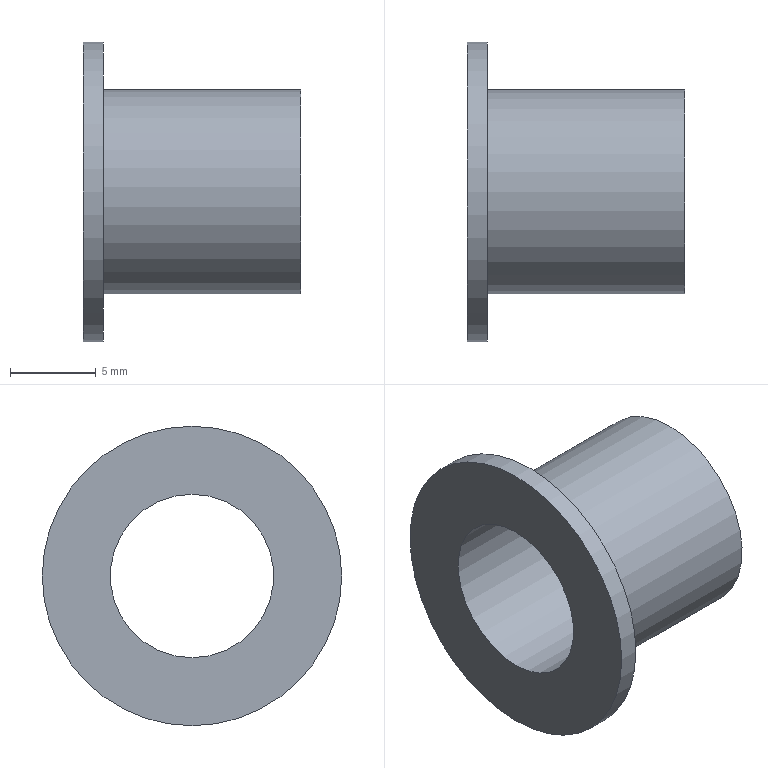Part | NX | features Igus GFI bushings(0.375 x 0.500) 2 | 1 solid | 6 faces | box 12.7 x 17.45 x 17.45 mm | volume 658.37 mm3 | plane 3 | cylinder 3 | commonest cylinder face diameters 9.525 x1 11.906 x1 17.45 x1
STEP:
#1=CARTESIAN_POINT('',(0.,0.,4.763));
#2=VERTEX_POINT('',#1);
#3=CARTESIAN_POINT('',(0.,0.,0.));
#4=DIRECTION('',(-1.,0.,0.));
#5=DIRECTION('',(0.,0.,1.));
#6=AXIS2_PLACEMENT_3D('',#3,#4,#5);
#7=CIRCLE('',#6,4.763);
#8=EDGE_CURVE('',#2,#2,#7,.T.);
#9=ORIENTED_EDGE('',*,*,#8,.F.);
#10=EDGE_LOOP('',(#9));
#11=FACE_BOUND('',#10,.T.);
#12=CARTESIAN_POINT('',(0.,0.,8.725));
#13=VERTEX_POINT('',#12);
#14=CARTESIAN_POINT('',(0.,0.,0.));
#15=DIRECTION('',(-1.,0.,0.));
#16=DIRECTION('',(0.,0.,1.));
#17=AXIS2_PLACEMENT_3D('',#14,#15,#16);
#18=CIRCLE('',#17,8.725);
#19=EDGE_CURVE('',#13,#13,#18,.T.);
#20=ORIENTED_EDGE('',*,*,#19,.T.);
#21=EDGE_LOOP('',(#20));
#22=FACE_BOUND('',#21,.T.);
#23=CARTESIAN_POINT('',(0.,4.763,0.));
#24=DIRECTION('',(1.,0.,0.));
#25=DIRECTION('',(0.,0.,-1.));
#26=AXIS2_PLACEMENT_3D('',#23,#24,#25);
#27=PLANE('',#26);
#28=ADVANCED_FACE('',(#11,#22),#27,.F.);
#29=CARTESIAN_POINT('',(12.7,0.,4.763));
#30=VERTEX_POINT('',#29);
#31=CARTESIAN_POINT('',(12.7,0.,0.));
#32=DIRECTION('',(-1.,0.,0.));
#33=DIRECTION('',(0.,0.,1.));
#34=AXIS2_PLACEMENT_3D('',#31,#32,#33);
#35=CIRCLE('',#34,4.763);
#36=EDGE_CURVE('',#30,#30,#35,.T.);
#37=ORIENTED_EDGE('',*,*,#36,.F.);
#38=EDGE_LOOP('',(#37));
#39=FACE_BOUND('',#38,.T.);
#40=ORIENTED_EDGE('',*,*,#8,.T.);
#41=EDGE_LOOP('',(#40));
#42=FACE_BOUND('',#41,.T.);
#43=CARTESIAN_POINT('',(0.,0.,0.));
#44=DIRECTION('',(-1.,0.,0.));
#45=DIRECTION('',(0.,0.,1.));
#46=AXIS2_PLACEMENT_3D('',#43,#44,#45);
#47=CYLINDRICAL_SURFACE('',#46,4.763);
#48=ADVANCED_FACE('',(#39,#42),#47,.F.);
#49=CARTESIAN_POINT('',(12.7,0.,5.953));
#50=VERTEX_POINT('',#49);
#51=CARTESIAN_POINT('',(12.7,0.,0.));
#52=DIRECTION('',(-1.,0.,0.));
#53=DIRECTION('',(0.,0.,1.));
#54=AXIS2_PLACEMENT_3D('',#51,#52,#53);
#55=CIRCLE('',#54,5.953);
#56=EDGE_CURVE('',#50,#50,#55,.T.);
#57=ORIENTED_EDGE('',*,*,#56,.F.);
#58=EDGE_LOOP('',(#57));
#59=FACE_BOUND('',#58,.T.);
#60=ORIENTED_EDGE('',*,*,#36,.T.);
#61=EDGE_LOOP('',(#60));
#62=FACE_BOUND('',#61,.T.);
#63=CARTESIAN_POINT('',(12.7,4.763,0.));
#64=DIRECTION('',(-1.,0.,0.));
#65=DIRECTION('',(0.,0.,1.));
#66=AXIS2_PLACEMENT_3D('',#63,#64,#65);
#67=PLANE('',#66);
#68=ADVANCED_FACE('',(#59,#62),#67,.F.);
#69=CARTESIAN_POINT('',(1.168,0.,5.953));
#70=VERTEX_POINT('',#69);
#71=CARTESIAN_POINT('',(1.168,0.,0.));
#72=DIRECTION('',(-1.,0.,0.));
#73=DIRECTION('',(0.,0.,1.));
#74=AXIS2_PLACEMENT_3D('',#71,#72,#73);
#75=CIRCLE('',#74,5.953);
#76=EDGE_CURVE('',#70,#70,#75,.T.);
#77=ORIENTED_EDGE('',*,*,#76,.F.);
#78=EDGE_LOOP('',(#77));
#79=FACE_BOUND('',#78,.T.);
#80=ORIENTED_EDGE('',*,*,#56,.T.);
#81=EDGE_LOOP('',(#80));
#82=FACE_BOUND('',#81,.T.);
#83=CARTESIAN_POINT('',(0.,0.,0.));
#84=DIRECTION('',(-1.,0.,0.));
#85=DIRECTION('',(0.,0.,1.));
#86=AXIS2_PLACEMENT_3D('',#83,#84,#85);
#87=CYLINDRICAL_SURFACE('',#86,5.953);
#88=ADVANCED_FACE('',(#79,#82),#87,.T.);
#89=CARTESIAN_POINT('',(1.168,0.,8.725));
#90=VERTEX_POINT('',#89);
#91=CARTESIAN_POINT('',(1.168,0.,0.));
#92=DIRECTION('',(-1.,0.,0.));
#93=DIRECTION('',(0.,0.,1.));
#94=AXIS2_PLACEMENT_3D('',#91,#92,#93);
#95=CIRCLE('',#94,8.725);
#96=EDGE_CURVE('',#90,#90,#95,.T.);
#97=ORIENTED_EDGE('',*,*,#96,.F.);
#98=EDGE_LOOP('',(#97));
#99=FACE_BOUND('',#98,.T.);
#100=ORIENTED_EDGE('',*,*,#76,.T.);
#101=EDGE_LOOP('',(#100));
#102=FACE_BOUND('',#101,.T.);
#103=CARTESIAN_POINT('',(1.168,5.953,0.));
#104=DIRECTION('',(-1.,0.,0.));
#105=DIRECTION('',(0.,0.,1.));
#106=AXIS2_PLACEMENT_3D('',#103,#104,#105);
#107=PLANE('',#106);
#108=ADVANCED_FACE('',(#99,#102),#107,.F.);
#109=ORIENTED_EDGE('',*,*,#19,.F.);
#110=EDGE_LOOP('',(#109));
#111=FACE_BOUND('',#110,.T.);
#112=ORIENTED_EDGE('',*,*,#96,.T.);
#113=EDGE_LOOP('',(#112));
#114=FACE_BOUND('',#113,.T.);
#115=CARTESIAN_POINT('',(0.,0.,0.));
#116=DIRECTION('',(-1.,0.,0.));
#117=DIRECTION('',(0.,0.,1.));
#118=AXIS2_PLACEMENT_3D('',#115,#116,#117);
#119=CYLINDRICAL_SURFACE('',#118,8.725);
#120=ADVANCED_FACE('',(#111,#114),#119,.T.);
#121=CLOSED_SHELL('',(#28,#48,#68,#88,#108,#120));
#122=MANIFOLD_SOLID_BREP('',#121);
#123=(LENGTH_UNIT()NAMED_UNIT(*)SI_UNIT(.MILLI.,.METRE.));
#124=UNCERTAINTY_MEASURE_WITH_UNIT(LENGTH_MEASURE(0.00001),#123,'','');
#125=(NAMED_UNIT(*)PLANE_ANGLE_UNIT()SI_UNIT($,.RADIAN.));
#126=(NAMED_UNIT(*)SI_UNIT($,.STERADIAN.)SOLID_ANGLE_UNIT());
#127=(GEOMETRIC_REPRESENTATION_CONTEXT(3)GLOBAL_UNCERTAINTY_ASSIGNED_CONTEXT((#124))GLOBAL_UNIT_ASSIGNED_CONTEXT((#123,#125,#126))REPRESENTATION_CONTEXT('',''));
#128=ADVANCED_BREP_SHAPE_REPRESENTATION('',(#122),#127);